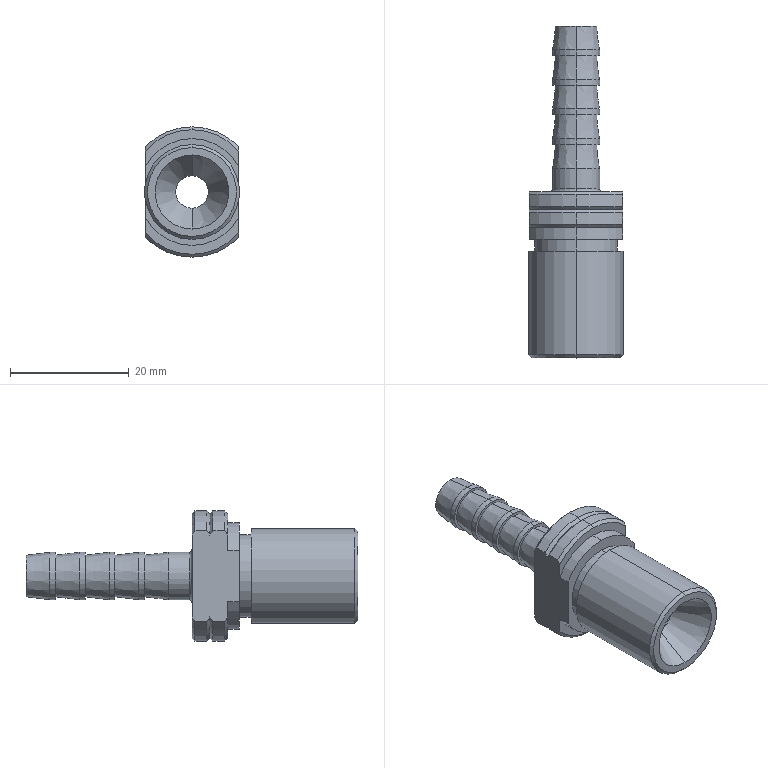Part | STEP file | HXGR200008-06-03-05 | 1 solid | 66 faces | box 16 x 56 x 22 mm | volume 5972 mm3 | cone 26 | cylinder 25 | plane 13 | torus 2 | commonest cylinder face diameters 8 x10 22 x6 18 x3 5.5 x2 14 x2 16 x2